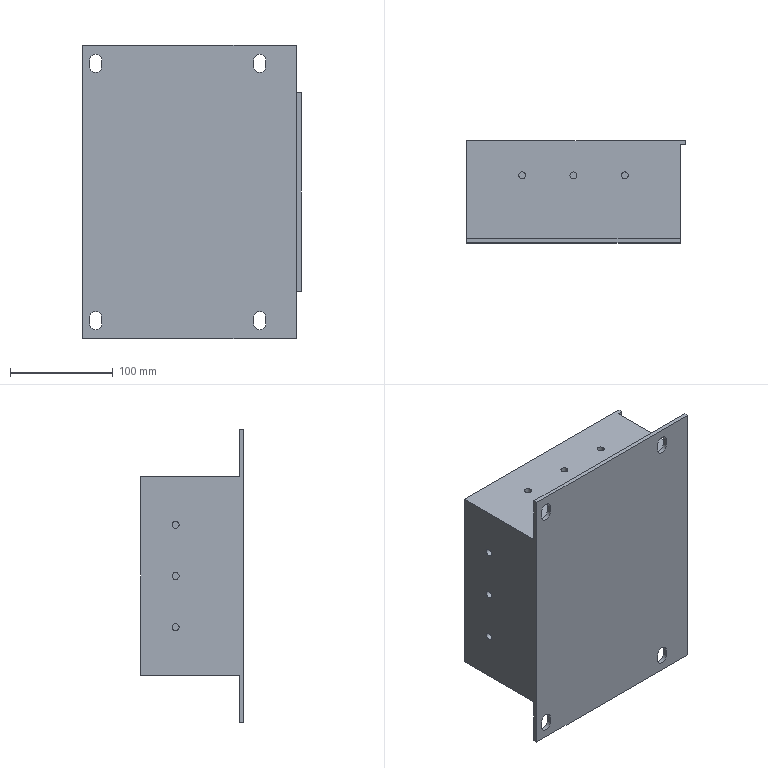Part | STEP file | a-hp_225_37-140_3_0_01 | 1 solid | 70 faces | box 213 x 100 x 286 mm | volume 4101760 mm3 | plane 41 | cylinder 29 | commonest cylinder face diameters 9 x12 6.8 x9 12 x8